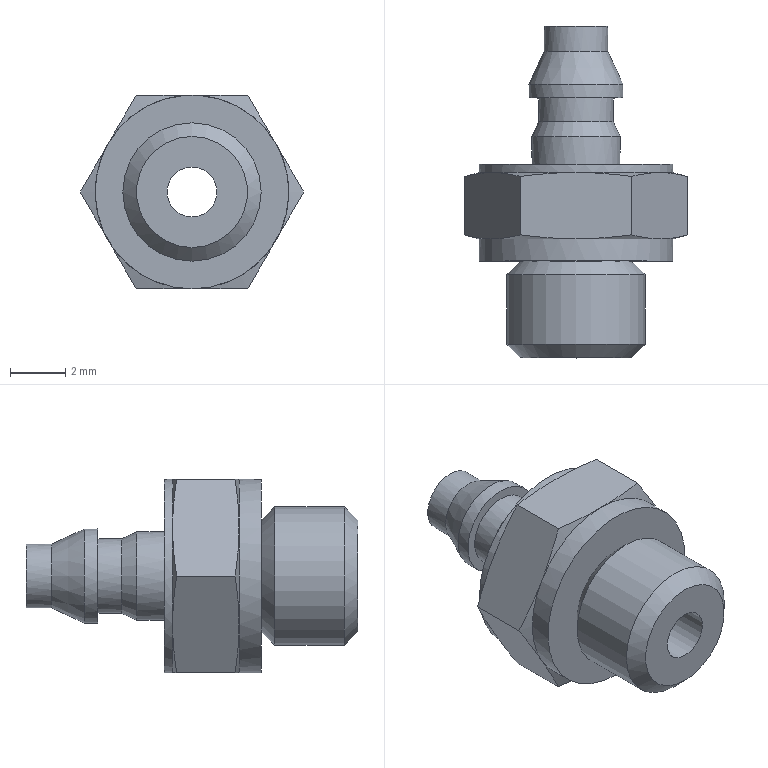Part | NX | 1 solid | 35 faces | box 8.083 x 12 x 7 mm | volume 211.126 mm3 | cone 16 | plane 11 | cylinder 8 | commonest cylinder face diameters 7 x2 1.8 x1 2.3 x1 2.7 x1 3.2 x1 3.4 x1
STEP:
#1=CARTESIAN_POINT('',(-3.031,3.2,-1.75));
#2=VERTEX_POINT('',#1);
#3=CARTESIAN_POINT('',(-3.031,3.2,1.75));
#4=VERTEX_POINT('',#3);
#5=CARTESIAN_POINT('',(0.,3.2,0.));
#6=DIRECTION('',(0.,-1.,0.));
#7=DIRECTION('',(-1.,0.,0.));
#8=AXIS2_PLACEMENT_3D('',#5,#6,#7);
#9=CIRCLE('',#8,3.5);
#10=EDGE_CURVE('',#2,#4,#9,.F.);
#11=ORIENTED_EDGE('',*,*,#10,.T.);
#12=CARTESIAN_POINT('',(0.,3.2,3.5));
#13=VERTEX_POINT('',#12);
#14=CARTESIAN_POINT('',(0.,3.2,0.));
#15=DIRECTION('',(0.,-1.,0.));
#16=DIRECTION('',(-1.,0.,0.));
#17=AXIS2_PLACEMENT_3D('',#14,#15,#16);
#18=CIRCLE('',#17,3.5);
#19=EDGE_CURVE('',#4,#13,#18,.F.);
#20=ORIENTED_EDGE('',*,*,#19,.T.);
#21=CARTESIAN_POINT('',(3.031,3.2,1.75));
#22=VERTEX_POINT('',#21);
#23=CARTESIAN_POINT('',(0.,3.2,0.));
#24=DIRECTION('',(0.,-1.,0.));
#25=DIRECTION('',(-1.,0.,0.));
#26=AXIS2_PLACEMENT_3D('',#23,#24,#25);
#27=CIRCLE('',#26,3.5);
#28=EDGE_CURVE('',#13,#22,#27,.F.);
#29=ORIENTED_EDGE('',*,*,#28,.T.);
#30=CARTESIAN_POINT('',(3.031,3.2,-1.75));
#31=VERTEX_POINT('',#30);
#32=CARTESIAN_POINT('',(0.,3.2,0.));
#33=DIRECTION('',(0.,-1.,0.));
#34=DIRECTION('',(-1.,0.,0.));
#35=AXIS2_PLACEMENT_3D('',#32,#33,#34);
#36=CIRCLE('',#35,3.5);
#37=EDGE_CURVE('',#22,#31,#36,.F.);
#38=ORIENTED_EDGE('',*,*,#37,.T.);
#39=CARTESIAN_POINT('',(0.,3.2,-3.5));
#40=VERTEX_POINT('',#39);
#41=CARTESIAN_POINT('',(0.,3.2,0.));
#42=DIRECTION('',(0.,-1.,0.));
#43=DIRECTION('',(-1.,0.,0.));
#44=AXIS2_PLACEMENT_3D('',#41,#42,#43);
#45=CIRCLE('',#44,3.5);
#46=EDGE_CURVE('',#31,#40,#45,.F.);
#47=ORIENTED_EDGE('',*,*,#46,.T.);
#48=CARTESIAN_POINT('',(0.,3.2,0.));
#49=DIRECTION('',(0.,-1.,0.));
#50=DIRECTION('',(-1.,0.,0.));
#51=AXIS2_PLACEMENT_3D('',#48,#49,#50);
#52=CIRCLE('',#51,3.5);
#53=EDGE_CURVE('',#40,#2,#52,.F.);
#54=ORIENTED_EDGE('',*,*,#53,.T.);
#55=EDGE_LOOP('',(#11,#20,#29,#38,#47,#54));
#56=FACE_BOUND('',#55,.T.);
#57=CARTESIAN_POINT('',(0.,3.5,-3.5));
#58=VERTEX_POINT('',#57);
#59=CARTESIAN_POINT('',(0.,3.5,0.));
#60=DIRECTION('',(0.,-1.,0.));
#61=DIRECTION('',(0.,0.,-1.));
#62=AXIS2_PLACEMENT_3D('',#59,#60,#61);
#63=CIRCLE('',#62,3.5);
#64=EDGE_CURVE('',#58,#58,#63,.T.);
#65=ORIENTED_EDGE('',*,*,#64,.T.);
#66=EDGE_LOOP('',(#65));
#67=FACE_BOUND('',#66,.T.);
#68=CARTESIAN_POINT('',(0.,3.2,0.));
#69=DIRECTION('',(0.,-1.,0.));
#70=DIRECTION('',(0.,0.,-1.));
#71=AXIS2_PLACEMENT_3D('',#68,#69,#70);
#72=CYLINDRICAL_SURFACE('',#71,3.5);
#73=ADVANCED_FACE('',(#56,#67),#72,.T.);
#74=ORIENTED_EDGE('',*,*,#10,.F.);
#75=CARTESIAN_POINT('',(-4.041,3.055,0.));
#76=VERTEX_POINT('',#75);
#77=CARTESIAN_POINT('',(-3.031,3.2,-1.75));
#78=CARTESIAN_POINT('',(-3.37,3.2,-1.164));
#79=CARTESIAN_POINT('',(-3.706,3.145,-0.5808));
#80=CARTESIAN_POINT('',(-4.041,3.055,0.));
#81=B_SPLINE_CURVE_WITH_KNOTS('',3,(#77,#78,#79,#80),.UNSPECIFIED.,.F.,.F.,(4,4),(0.,0.002026),.UNSPECIFIED.);
#82=EDGE_CURVE('',#2,#76,#81,.T.);
#83=ORIENTED_EDGE('',*,*,#82,.T.);
#84=CARTESIAN_POINT('',(-3.031,3.2,1.75));
#85=CARTESIAN_POINT('',(-3.37,3.2,1.164));
#86=CARTESIAN_POINT('',(-3.706,3.145,0.5808));
#87=CARTESIAN_POINT('',(-4.041,3.055,0.));
#88=B_SPLINE_CURVE_WITH_KNOTS('',3,(#84,#85,#86,#87),.UNSPECIFIED.,.F.,.F.,(4,4),(0.,0.002026),.UNSPECIFIED.);
#89=EDGE_CURVE('',#4,#76,#88,.T.);
#90=ORIENTED_EDGE('',*,*,#89,.F.);
#91=EDGE_LOOP('',(#74,#83,#90));
#92=FACE_BOUND('',#91,.T.);
#93=CARTESIAN_POINT('',(0.,3.2,0.));
#94=DIRECTION('',(0.,-1.,0.));
#95=DIRECTION('',(0.,0.,-1.));
#96=AXIS2_PLACEMENT_3D('',#93,#94,#95);
#97=CONICAL_SURFACE('',#96,3.5,1.309);
#98=ADVANCED_FACE('',(#92),#97,.T.);
#99=CARTESIAN_POINT('',(-2.021,3.055,-3.5));
#100=VERTEX_POINT('',#99);
#101=CARTESIAN_POINT('',(-2.021,3.055,-3.5));
#102=CARTESIAN_POINT('',(-2.356,3.145,-2.919));
#103=CARTESIAN_POINT('',(-2.693,3.2,-2.336));
#104=CARTESIAN_POINT('',(-3.031,3.2,-1.75));
#105=B_SPLINE_CURVE_WITH_KNOTS('',3,(#101,#102,#103,#104),.UNSPECIFIED.,.F.,.F.,(4,4),(0.,0.002026),.UNSPECIFIED.);
#106=EDGE_CURVE('',#100,#2,#105,.T.);
#107=ORIENTED_EDGE('',*,*,#106,.T.);
#108=ORIENTED_EDGE('',*,*,#53,.F.);
#109=CARTESIAN_POINT('',(0.,3.2,-3.5));
#110=CARTESIAN_POINT('',(-0.677,3.2,-3.5));
#111=CARTESIAN_POINT('',(-1.35,3.145,-3.5));
#112=CARTESIAN_POINT('',(-2.021,3.055,-3.5));
#113=B_SPLINE_CURVE_WITH_KNOTS('',3,(#109,#110,#111,#112),.UNSPECIFIED.,.F.,.F.,(4,4),(0.,0.002026),.UNSPECIFIED.);
#114=EDGE_CURVE('',#40,#100,#113,.T.);
#115=ORIENTED_EDGE('',*,*,#114,.T.);
#116=EDGE_LOOP('',(#107,#108,#115));
#117=FACE_BOUND('',#116,.T.);
#118=CARTESIAN_POINT('',(0.,3.2,0.));
#119=DIRECTION('',(0.,-1.,0.));
#120=DIRECTION('',(0.,0.,-1.));
#121=AXIS2_PLACEMENT_3D('',#118,#119,#120);
#122=CONICAL_SURFACE('',#121,3.5,1.309);
#123=ADVANCED_FACE('',(#117),#122,.T.);
#124=CARTESIAN_POINT('',(2.021,3.055,-3.5));
#125=VERTEX_POINT('',#124);
#126=CARTESIAN_POINT('',(2.021,3.055,-3.5));
#127=CARTESIAN_POINT('',(1.35,3.145,-3.5));
#128=CARTESIAN_POINT('',(0.677,3.2,-3.5));
#129=CARTESIAN_POINT('',(0.,3.2,-3.5));
#130=B_SPLINE_CURVE_WITH_KNOTS('',3,(#126,#127,#128,#129),.UNSPECIFIED.,.F.,.F.,(4,4),(0.,0.002026),.UNSPECIFIED.);
#131=EDGE_CURVE('',#125,#40,#130,.T.);
#132=ORIENTED_EDGE('',*,*,#131,.T.);
#133=ORIENTED_EDGE('',*,*,#46,.F.);
#134=CARTESIAN_POINT('',(3.031,3.2,-1.75));
#135=CARTESIAN_POINT('',(2.693,3.2,-2.336));
#136=CARTESIAN_POINT('',(2.356,3.145,-2.919));
#137=CARTESIAN_POINT('',(2.021,3.055,-3.5));
#138=B_SPLINE_CURVE_WITH_KNOTS('',3,(#134,#135,#136,#137),.UNSPECIFIED.,.F.,.F.,(4,4),(0.,0.002026),.UNSPECIFIED.);
#139=EDGE_CURVE('',#31,#125,#138,.T.);
#140=ORIENTED_EDGE('',*,*,#139,.T.);
#141=EDGE_LOOP('',(#132,#133,#140));
#142=FACE_BOUND('',#141,.T.);
#143=CARTESIAN_POINT('',(0.,3.2,0.));
#144=DIRECTION('',(0.,-1.,0.));
#145=DIRECTION('',(0.,0.,-1.));
#146=AXIS2_PLACEMENT_3D('',#143,#144,#145);
#147=CONICAL_SURFACE('',#146,3.5,1.309);
#148=ADVANCED_FACE('',(#142),#147,.T.);
#149=CARTESIAN_POINT('',(4.041,3.055,0.));
#150=VERTEX_POINT('',#149);
#151=CARTESIAN_POINT('',(4.041,3.055,0.));
#152=CARTESIAN_POINT('',(3.706,3.145,-0.5808));
#153=CARTESIAN_POINT('',(3.37,3.2,-1.164));
#154=CARTESIAN_POINT('',(3.031,3.2,-1.75));
#155=B_SPLINE_CURVE_WITH_KNOTS('',3,(#151,#152,#153,#154),.UNSPECIFIED.,.F.,.F.,(4,4),(0.,0.002026),.UNSPECIFIED.);
#156=EDGE_CURVE('',#150,#31,#155,.T.);
#157=ORIENTED_EDGE('',*,*,#156,.T.);
#158=ORIENTED_EDGE('',*,*,#37,.F.);
#159=CARTESIAN_POINT('',(4.041,3.055,0.));
#160=CARTESIAN_POINT('',(3.706,3.145,0.5808));
#161=CARTESIAN_POINT('',(3.37,3.2,1.164));
#162=CARTESIAN_POINT('',(3.031,3.2,1.75));
#163=B_SPLINE_CURVE_WITH_KNOTS('',3,(#159,#160,#161,#162),.UNSPECIFIED.,.F.,.F.,(4,4),(0.,0.002026),.UNSPECIFIED.);
#164=EDGE_CURVE('',#150,#22,#163,.T.);
#165=ORIENTED_EDGE('',*,*,#164,.F.);
#166=EDGE_LOOP('',(#157,#158,#165));
#167=FACE_BOUND('',#166,.T.);
#168=CARTESIAN_POINT('',(0.,3.2,0.));
#169=DIRECTION('',(0.,-1.,0.));
#170=DIRECTION('',(0.,0.,-1.));
#171=AXIS2_PLACEMENT_3D('',#168,#169,#170);
#172=CONICAL_SURFACE('',#171,3.5,1.309);
#173=ADVANCED_FACE('',(#167),#172,.T.);
#174=CARTESIAN_POINT('',(0.,3.5,-1.6));
#175=VERTEX_POINT('',#174);
#176=CARTESIAN_POINT('',(0.,3.5,0.));
#177=DIRECTION('',(0.,-1.,0.));
#178=DIRECTION('',(0.,0.,-1.));
#179=AXIS2_PLACEMENT_3D('',#176,#177,#178);
#180=CIRCLE('',#179,1.6);
#181=EDGE_CURVE('',#175,#175,#180,.T.);
#182=ORIENTED_EDGE('',*,*,#181,.T.);
#183=EDGE_LOOP('',(#182));
#184=FACE_BOUND('',#183,.T.);
#185=ORIENTED_EDGE('',*,*,#64,.F.);
#186=EDGE_LOOP('',(#185));
#187=FACE_BOUND('',#186,.T.);
#188=CARTESIAN_POINT('',(-3.5,3.5,3.542));
#189=DIRECTION('',(0.,1.,0.));
#190=DIRECTION('',(1.,0.,0.));
#191=AXIS2_PLACEMENT_3D('',#188,#189,#190);
#192=PLANE('',#191);
#193=ADVANCED_FACE('',(#184,#187),#192,.T.);
#194=CARTESIAN_POINT('',(-4.041,0.9451,0.));
#195=VERTEX_POINT('',#194);
#196=CARTESIAN_POINT('',(-4.041,0.8,0.));
#197=DIRECTION('',(0.,1.,0.));
#198=VECTOR('',#197,1000.);
#199=LINE('',#196,#198);
#200=EDGE_CURVE('',#195,#76,#199,.T.);
#201=ORIENTED_EDGE('',*,*,#200,.T.);
#202=ORIENTED_EDGE('',*,*,#82,.F.);
#203=ORIENTED_EDGE('',*,*,#106,.F.);
#204=CARTESIAN_POINT('',(-2.021,0.9451,-3.5));
#205=VERTEX_POINT('',#204);
#206=CARTESIAN_POINT('',(-2.021,0.8,-3.5));
#207=DIRECTION('',(0.,1.,0.));
#208=VECTOR('',#207,1000.);
#209=LINE('',#206,#208);
#210=EDGE_CURVE('',#100,#205,#209,.F.);
#211=ORIENTED_EDGE('',*,*,#210,.T.);
#212=CARTESIAN_POINT('',(-3.031,0.8,-1.75));
#213=VERTEX_POINT('',#212);
#214=CARTESIAN_POINT('',(-2.021,0.9451,-3.5));
#215=CARTESIAN_POINT('',(-2.356,0.8552,-2.919));
#216=CARTESIAN_POINT('',(-2.693,0.8,-2.336));
#217=CARTESIAN_POINT('',(-3.031,0.8,-1.75));
#218=B_SPLINE_CURVE_WITH_KNOTS('',3,(#214,#215,#216,#217),.UNSPECIFIED.,.F.,.F.,(4,4),(0.,0.002026),.UNSPECIFIED.);
#219=EDGE_CURVE('',#205,#213,#218,.T.);
#220=ORIENTED_EDGE('',*,*,#219,.T.);
#221=CARTESIAN_POINT('',(-3.031,0.8,-1.75));
#222=CARTESIAN_POINT('',(-3.37,0.8,-1.164));
#223=CARTESIAN_POINT('',(-3.706,0.8552,-0.5808));
#224=CARTESIAN_POINT('',(-4.041,0.9451,0.));
#225=B_SPLINE_CURVE_WITH_KNOTS('',3,(#221,#222,#223,#224),.UNSPECIFIED.,.F.,.F.,(4,4),(0.,0.002026),.UNSPECIFIED.);
#226=EDGE_CURVE('',#213,#195,#225,.T.);
#227=ORIENTED_EDGE('',*,*,#226,.T.);
#228=EDGE_LOOP('',(#201,#202,#203,#211,#220,#227));
#229=FACE_BOUND('',#228,.T.);
#230=CARTESIAN_POINT('',(-2.021,0.7856,-3.5));
#231=DIRECTION('',(-0.866,0.,-0.5));
#232=DIRECTION('',(-0.5,0.,0.866));
#233=AXIS2_PLACEMENT_3D('',#230,#231,#232);
#234=PLANE('',#233);
#235=ADVANCED_FACE('',(#229),#234,.T.);
#236=ORIENTED_EDGE('',*,*,#210,.F.);
#237=ORIENTED_EDGE('',*,*,#114,.F.);
#238=ORIENTED_EDGE('',*,*,#131,.F.);
#239=CARTESIAN_POINT('',(2.021,0.9451,-3.5));
#240=VERTEX_POINT('',#239);
#241=CARTESIAN_POINT('',(2.021,0.8,-3.5));
#242=DIRECTION('',(0.,1.,0.));
#243=VECTOR('',#242,1000.);
#244=LINE('',#241,#243);
#245=EDGE_CURVE('',#125,#240,#244,.F.);
#246=ORIENTED_EDGE('',*,*,#245,.T.);
#247=CARTESIAN_POINT('',(0.,0.8,-3.5));
#248=VERTEX_POINT('',#247);
#249=CARTESIAN_POINT('',(2.021,0.9451,-3.5));
#250=CARTESIAN_POINT('',(1.35,0.8552,-3.5));
#251=CARTESIAN_POINT('',(0.677,0.8,-3.5));
#252=CARTESIAN_POINT('',(0.,0.8,-3.5));
#253=B_SPLINE_CURVE_WITH_KNOTS('',3,(#249,#250,#251,#252),.UNSPECIFIED.,.F.,.F.,(4,4),(0.,0.002026),.UNSPECIFIED.);
#254=EDGE_CURVE('',#240,#248,#253,.T.);
#255=ORIENTED_EDGE('',*,*,#254,.T.);
#256=CARTESIAN_POINT('',(0.,0.8,-3.5));
#257=CARTESIAN_POINT('',(-0.677,0.8,-3.5));
#258=CARTESIAN_POINT('',(-1.35,0.8552,-3.5));
#259=CARTESIAN_POINT('',(-2.021,0.9451,-3.5));
#260=B_SPLINE_CURVE_WITH_KNOTS('',3,(#256,#257,#258,#259),.UNSPECIFIED.,.F.,.F.,(4,4),(0.,0.002026),.UNSPECIFIED.);
#261=EDGE_CURVE('',#248,#205,#260,.T.);
#262=ORIENTED_EDGE('',*,*,#261,.T.);
#263=EDGE_LOOP('',(#236,#237,#238,#246,#255,#262));
#264=FACE_BOUND('',#263,.T.);
#265=CARTESIAN_POINT('',(2.021,0.7856,-3.5));
#266=DIRECTION('',(0.,0.,-1.));
#267=DIRECTION('',(-1.,0.,0.));
#268=AXIS2_PLACEMENT_3D('',#265,#266,#267);
#269=PLANE('',#268);
#270=ADVANCED_FACE('',(#264),#269,.T.);
#271=ORIENTED_EDGE('',*,*,#245,.F.);
#272=ORIENTED_EDGE('',*,*,#139,.F.);
#273=ORIENTED_EDGE('',*,*,#156,.F.);
#274=CARTESIAN_POINT('',(4.041,0.9451,0.));
#275=VERTEX_POINT('',#274);
#276=CARTESIAN_POINT('',(4.041,0.8,0.));
#277=DIRECTION('',(0.,1.,0.));
#278=VECTOR('',#277,1000.);
#279=LINE('',#276,#278);
#280=EDGE_CURVE('',#150,#275,#279,.F.);
#281=ORIENTED_EDGE('',*,*,#280,.T.);
#282=CARTESIAN_POINT('',(3.031,0.8,-1.75));
#283=VERTEX_POINT('',#282);
#284=CARTESIAN_POINT('',(4.041,0.9451,0.));
#285=CARTESIAN_POINT('',(3.706,0.8552,-0.5808));
#286=CARTESIAN_POINT('',(3.37,0.8,-1.164));
#287=CARTESIAN_POINT('',(3.031,0.8,-1.75));
#288=B_SPLINE_CURVE_WITH_KNOTS('',3,(#284,#285,#286,#287),.UNSPECIFIED.,.F.,.F.,(4,4),(0.,0.002026),.UNSPECIFIED.);
#289=EDGE_CURVE('',#275,#283,#288,.T.);
#290=ORIENTED_EDGE('',*,*,#289,.T.);
#291=CARTESIAN_POINT('',(3.031,0.8,-1.75));
#292=CARTESIAN_POINT('',(2.693,0.8,-2.336));
#293=CARTESIAN_POINT('',(2.356,0.8552,-2.919));
#294=CARTESIAN_POINT('',(2.021,0.9451,-3.5));
#295=B_SPLINE_CURVE_WITH_KNOTS('',3,(#291,#292,#293,#294),.UNSPECIFIED.,.F.,.F.,(4,4),(0.,0.002026),.UNSPECIFIED.);
#296=EDGE_CURVE('',#283,#240,#295,.T.);
#297=ORIENTED_EDGE('',*,*,#296,.T.);
#298=EDGE_LOOP('',(#271,#272,#273,#281,#290,#297));
#299=FACE_BOUND('',#298,.T.);
#300=CARTESIAN_POINT('',(4.041,0.7856,0.));
#301=DIRECTION('',(0.866,0.,-0.5));
#302=DIRECTION('',(-0.5,0.,-0.866));
#303=AXIS2_PLACEMENT_3D('',#300,#301,#302);
#304=PLANE('',#303);
#305=ADVANCED_FACE('',(#299),#304,.T.);
#306=ORIENTED_EDGE('',*,*,#181,.F.);
#307=EDGE_LOOP('',(#306));
#308=FACE_BOUND('',#307,.T.);
#309=CARTESIAN_POINT('',(-1.6,4.5,0.));
#310=VERTEX_POINT('',#309);
#311=CARTESIAN_POINT('',(0.,4.5,0.));
#312=DIRECTION('',(0.,-1.,0.));
#313=DIRECTION('',(-1.,0.,0.));
#314=AXIS2_PLACEMENT_3D('',#311,#312,#313);
#315=CIRCLE('',#314,1.6);
#316=EDGE_CURVE('',#310,#310,#315,.T.);
#317=ORIENTED_EDGE('',*,*,#316,.T.);
#318=EDGE_LOOP('',(#317));
#319=FACE_BOUND('',#318,.T.);
#320=CARTESIAN_POINT('',(0.,3.5,0.));
#321=DIRECTION('',(0.,-1.,0.));
#322=DIRECTION('',(0.,0.,-1.));
#323=AXIS2_PLACEMENT_3D('',#320,#321,#322);
#324=CYLINDRICAL_SURFACE('',#323,1.6);
#325=ADVANCED_FACE('',(#308,#319),#324,.T.);
#326=CARTESIAN_POINT('',(-3.031,0.8,1.75));
#327=VERTEX_POINT('',#326);
#328=CARTESIAN_POINT('',(-2.021,0.9451,3.5));
#329=VERTEX_POINT('',#328);
#330=CARTESIAN_POINT('',(-3.031,0.8,1.75));
#331=CARTESIAN_POINT('',(-2.693,0.8,2.336));
#332=CARTESIAN_POINT('',(-2.356,0.8552,2.919));
#333=CARTESIAN_POINT('',(-2.021,0.9451,3.5));
#334=B_SPLINE_CURVE_WITH_KNOTS('',3,(#330,#331,#332,#333),.UNSPECIFIED.,.F.,.F.,(4,4),(0.,0.002026),.UNSPECIFIED.);
#335=EDGE_CURVE('',#327,#329,#334,.T.);
#336=ORIENTED_EDGE('',*,*,#335,.T.);
#337=CARTESIAN_POINT('',(-2.021,3.055,3.5));
#338=VERTEX_POINT('',#337);
#339=CARTESIAN_POINT('',(-2.021,0.8,3.5));
#340=DIRECTION('',(0.,1.,0.));
#341=VECTOR('',#340,1000.);
#342=LINE('',#339,#341);
#343=EDGE_CURVE('',#329,#338,#342,.T.);
#344=ORIENTED_EDGE('',*,*,#343,.T.);
#345=CARTESIAN_POINT('',(-2.021,3.055,3.5));
#346=CARTESIAN_POINT('',(-2.356,3.145,2.919));
#347=CARTESIAN_POINT('',(-2.693,3.2,2.336));
#348=CARTESIAN_POINT('',(-3.031,3.2,1.75));
#349=B_SPLINE_CURVE_WITH_KNOTS('',3,(#345,#346,#347,#348),.UNSPECIFIED.,.F.,.F.,(4,4),(0.,0.002026),.UNSPECIFIED.);
#350=EDGE_CURVE('',#338,#4,#349,.T.);
#351=ORIENTED_EDGE('',*,*,#350,.T.);
#352=ORIENTED_EDGE('',*,*,#89,.T.);
#353=ORIENTED_EDGE('',*,*,#200,.F.);
#354=CARTESIAN_POINT('',(-4.041,0.9451,0.));
#355=CARTESIAN_POINT('',(-3.706,0.8552,0.5808));
#356=CARTESIAN_POINT('',(-3.37,0.8,1.164));
#357=CARTESIAN_POINT('',(-3.031,0.8,1.75));
#358=B_SPLINE_CURVE_WITH_KNOTS('',3,(#354,#355,#356,#357),.UNSPECIFIED.,.F.,.F.,(4,4),(0.,0.002026),.UNSPECIFIED.);
#359=EDGE_CURVE('',#195,#327,#358,.T.);
#360=ORIENTED_EDGE('',*,*,#359,.T.);
#361=EDGE_LOOP('',(#336,#344,#351,#352,#353,#360));
#362=FACE_BOUND('',#361,.T.);
#363=CARTESIAN_POINT('',(-4.041,0.7856,0.));
#364=DIRECTION('',(-0.866,0.,0.5));
#365=DIRECTION('',(0.5,0.,0.866));
#366=AXIS2_PLACEMENT_3D('',#363,#364,#365);
#367=PLANE('',#366);
#368=ADVANCED_FACE('',(#362),#367,.T.);
#369=ORIENTED_EDGE('',*,*,#226,.F.);
#370=CARTESIAN_POINT('',(0.,0.8,0.));
#371=DIRECTION('',(0.,-1.,0.));
#372=DIRECTION('',(-1.,0.,0.));
#373=AXIS2_PLACEMENT_3D('',#370,#371,#372);
#374=CIRCLE('',#373,3.5);
#375=EDGE_CURVE('',#213,#327,#374,.F.);
#376=ORIENTED_EDGE('',*,*,#375,.T.);
#377=ORIENTED_EDGE('',*,*,#359,.F.);
#378=EDGE_LOOP('',(#369,#376,#377));
#379=FACE_BOUND('',#378,.T.);
#380=CARTESIAN_POINT('',(0.,0.8,0.));
#381=DIRECTION('',(0.,1.,0.));
#382=DIRECTION('',(0.,0.,1.));
#383=AXIS2_PLACEMENT_3D('',#380,#381,#382);
#384=CONICAL_SURFACE('',#383,3.5,1.309);
#385=ADVANCED_FACE('',(#379),#384,.T.);
#386=ORIENTED_EDGE('',*,*,#261,.F.);
#387=CARTESIAN_POINT('',(0.,0.8,0.));
#388=DIRECTION('',(0.,-1.,0.));
#389=DIRECTION('',(-1.,0.,0.));
#390=AXIS2_PLACEMENT_3D('',#387,#388,#389);
#391=CIRCLE('',#390,3.5);
#392=EDGE_CURVE('',#248,#213,#391,.F.);
#393=ORIENTED_EDGE('',*,*,#392,.T.);
#394=ORIENTED_EDGE('',*,*,#219,.F.);
#395=EDGE_LOOP('',(#386,#393,#394));
#396=FACE_BOUND('',#395,.T.);
#397=CARTESIAN_POINT('',(0.,0.8,0.));
#398=DIRECTION('',(0.,1.,0.));
#399=DIRECTION('',(0.,0.,1.));
#400=AXIS2_PLACEMENT_3D('',#397,#398,#399);
#401=CONICAL_SURFACE('',#400,3.5,1.309);
#402=ADVANCED_FACE('',(#396),#401,.T.);
#403=CARTESIAN_POINT('',(0.,0.8,0.));
#404=DIRECTION('',(0.,-1.,0.));
#405=DIRECTION('',(-1.,0.,0.));
#406=AXIS2_PLACEMENT_3D('',#403,#404,#405);
#407=CIRCLE('',#406,3.5);
#408=EDGE_CURVE('',#283,#248,#407,.F.);
#409=ORIENTED_EDGE('',*,*,#408,.T.);
#410=ORIENTED_EDGE('',*,*,#254,.F.);
#411=ORIENTED_EDGE('',*,*,#296,.F.);
#412=EDGE_LOOP('',(#409,#410,#411));
#413=FACE_BOUND('',#412,.T.);
#414=CARTESIAN_POINT('',(0.,0.8,0.));
#415=DIRECTION('',(0.,1.,0.));
#416=DIRECTION('',(0.,0.,1.));
#417=AXIS2_PLACEMENT_3D('',#414,#415,#416);
#418=CONICAL_SURFACE('',#417,3.5,1.309);
#419=ADVANCED_FACE('',(#413),#418,.T.);
#420=CARTESIAN_POINT('',(3.031,0.8,1.75));
#421=VERTEX_POINT('',#420);
#422=CARTESIAN_POINT('',(0.,0.8,0.));
#423=DIRECTION('',(0.,-1.,0.));
#424=DIRECTION('',(-1.,0.,0.));
#425=AXIS2_PLACEMENT_3D('',#422,#423,#424);
#426=CIRCLE('',#425,3.5);
#427=EDGE_CURVE('',#421,#283,#426,.F.);
#428=ORIENTED_EDGE('',*,*,#427,.T.);
#429=ORIENTED_EDGE('',*,*,#289,.F.);
#430=CARTESIAN_POINT('',(3.031,0.8,1.75));
#431=CARTESIAN_POINT('',(3.37,0.8,1.164));
#432=CARTESIAN_POINT('',(3.706,0.8552,0.5808));
#433=CARTESIAN_POINT('',(4.041,0.9451,0.));
#434=B_SPLINE_CURVE_WITH_KNOTS('',3,(#430,#431,#432,#433),.UNSPECIFIED.,.F.,.F.,(4,4),(0.,0.002026),.UNSPECIFIED.);
#435=EDGE_CURVE('',#421,#275,#434,.T.);
#436=ORIENTED_EDGE('',*,*,#435,.F.);
#437=EDGE_LOOP('',(#428,#429,#436));
#438=FACE_BOUND('',#437,.T.);
#439=CARTESIAN_POINT('',(0.,0.8,0.));
#440=DIRECTION('',(0.,1.,0.));
#441=DIRECTION('',(0.,0.,1.));
#442=AXIS2_PLACEMENT_3D('',#439,#440,#441);
#443=CONICAL_SURFACE('',#442,3.5,1.309);
#444=ADVANCED_FACE('',(#438),#443,.T.);
#445=ORIENTED_EDGE('',*,*,#435,.T.);
#446=ORIENTED_EDGE('',*,*,#280,.F.);
#447=ORIENTED_EDGE('',*,*,#164,.T.);
#448=CARTESIAN_POINT('',(2.021,3.055,3.5));
#449=VERTEX_POINT('',#448);
#450=CARTESIAN_POINT('',(3.031,3.2,1.75));
#451=CARTESIAN_POINT('',(2.693,3.2,2.336));
#452=CARTESIAN_POINT('',(2.356,3.145,2.919));
#453=CARTESIAN_POINT('',(2.021,3.055,3.5));
#454=B_SPLINE_CURVE_WITH_KNOTS('',3,(#450,#451,#452,#453),.UNSPECIFIED.,.F.,.F.,(4,4),(0.,0.002026),.UNSPECIFIED.);
#455=EDGE_CURVE('',#22,#449,#454,.T.);
#456=ORIENTED_EDGE('',*,*,#455,.T.);
#457=CARTESIAN_POINT('',(2.021,0.9451,3.5));
#458=VERTEX_POINT('',#457);
#459=CARTESIAN_POINT('',(2.021,0.8,3.5));
#460=DIRECTION('',(0.,1.,0.));
#461=VECTOR('',#460,1000.);
#462=LINE('',#459,#461);
#463=EDGE_CURVE('',#449,#458,#462,.F.);
#464=ORIENTED_EDGE('',*,*,#463,.T.);
#465=CARTESIAN_POINT('',(2.021,0.9451,3.5));
#466=CARTESIAN_POINT('',(2.356,0.8552,2.919));
#467=CARTESIAN_POINT('',(2.693,0.8,2.336));
#468=CARTESIAN_POINT('',(3.031,0.8,1.75));
#469=B_SPLINE_CURVE_WITH_KNOTS('',3,(#465,#466,#467,#468),.UNSPECIFIED.,.F.,.F.,(4,4),(0.,0.002026),.UNSPECIFIED.);
#470=EDGE_CURVE('',#458,#421,#469,.T.);
#471=ORIENTED_EDGE('',*,*,#470,.T.);
#472=EDGE_LOOP('',(#445,#446,#447,#456,#464,#471));
#473=FACE_BOUND('',#472,.T.);
#474=CARTESIAN_POINT('',(2.021,0.7856,3.5));
#475=DIRECTION('',(0.866,0.,0.5));
#476=DIRECTION('',(0.5,0.,-0.866));
#477=AXIS2_PLACEMENT_3D('',#474,#475,#476);
#478=PLANE('',#477);
#479=ADVANCED_FACE('',(#473),#478,.T.);
#480=ORIENTED_EDGE('',*,*,#316,.F.);
#481=EDGE_LOOP('',(#480));
#482=FACE_BOUND('',#481,.T.);
#483=CARTESIAN_POINT('',(-1.35,5.04,0.));
#484=VERTEX_POINT('',#483);
#485=CARTESIAN_POINT('',(0.,5.04,0.));
#486=DIRECTION('',(0.,1.,0.));
#487=DIRECTION('',(-1.,0.,0.));
#488=AXIS2_PLACEMENT_3D('',#485,#486,#487);
#489=CIRCLE('',#488,1.35);
#490=EDGE_CURVE('',#484,#484,#489,.F.);
#491=ORIENTED_EDGE('',*,*,#490,.T.);
#492=EDGE_LOOP('',(#491));
#493=FACE_BOUND('',#492,.T.);
#494=CARTESIAN_POINT('',(0.,5.04,0.));
#495=DIRECTION('',(0.,-1.,0.));
#496=DIRECTION('',(0.,0.,-1.));
#497=AXIS2_PLACEMENT_3D('',#494,#495,#496);
#498=CONICAL_SURFACE('',#497,1.35,0.4336);
#499=ADVANCED_FACE('',(#482,#493),#498,.T.);
#500=ORIENTED_EDGE('',*,*,#28,.F.);
#501=CARTESIAN_POINT('',(0.,3.2,3.5));
#502=CARTESIAN_POINT('',(0.677,3.2,3.5));
#503=CARTESIAN_POINT('',(1.35,3.145,3.5));
#504=CARTESIAN_POINT('',(2.021,3.055,3.5));
#505=B_SPLINE_CURVE_WITH_KNOTS('',3,(#501,#502,#503,#504),.UNSPECIFIED.,.F.,.F.,(4,4),(0.,0.002026),.UNSPECIFIED.);
#506=EDGE_CURVE('',#13,#449,#505,.T.);
#507=ORIENTED_EDGE('',*,*,#506,.T.);
#508=ORIENTED_EDGE('',*,*,#455,.F.);
#509=EDGE_LOOP('',(#500,#507,#508));
#510=FACE_BOUND('',#509,.T.);
#511=CARTESIAN_POINT('',(0.,3.2,0.));
#512=DIRECTION('',(0.,-1.,0.));
#513=DIRECTION('',(0.,0.,-1.));
#514=AXIS2_PLACEMENT_3D('',#511,#512,#513);
#515=CONICAL_SURFACE('',#514,3.5,1.309);
#516=ADVANCED_FACE('',(#510),#515,.T.);
#517=ORIENTED_EDGE('',*,*,#19,.F.);
#518=ORIENTED_EDGE('',*,*,#350,.F.);
#519=CARTESIAN_POINT('',(-2.021,3.055,3.5));
#520=CARTESIAN_POINT('',(-1.35,3.145,3.5));
#521=CARTESIAN_POINT('',(-0.677,3.2,3.5));
#522=CARTESIAN_POINT('',(0.,3.2,3.5));
#523=B_SPLINE_CURVE_WITH_KNOTS('',3,(#519,#520,#521,#522),.UNSPECIFIED.,.F.,.F.,(4,4),(0.,0.002026),.UNSPECIFIED.);
#524=EDGE_CURVE('',#338,#13,#523,.T.);
#525=ORIENTED_EDGE('',*,*,#524,.T.);
#526=EDGE_LOOP('',(#517,#518,#525));
#527=FACE_BOUND('',#526,.T.);
#528=CARTESIAN_POINT('',(0.,3.2,0.));
#529=DIRECTION('',(0.,-1.,0.));
#530=DIRECTION('',(0.,0.,-1.));
#531=AXIS2_PLACEMENT_3D('',#528,#529,#530);
#532=CONICAL_SURFACE('',#531,3.5,1.309);
#533=ADVANCED_FACE('',(#527),#532,.T.);
#534=CARTESIAN_POINT('',(0.,0.8,3.5));
#535=VERTEX_POINT('',#534);
#536=CARTESIAN_POINT('',(0.,0.8,3.5));
#537=CARTESIAN_POINT('',(0.677,0.8,3.5));
#538=CARTESIAN_POINT('',(1.35,0.8552,3.5));
#539=CARTESIAN_POINT('',(2.021,0.9451,3.5));
#540=B_SPLINE_CURVE_WITH_KNOTS('',3,(#536,#537,#538,#539),.UNSPECIFIED.,.F.,.F.,(4,4),(0.,0.002026),.UNSPECIFIED.);
#541=EDGE_CURVE('',#535,#458,#540,.T.);
#542=ORIENTED_EDGE('',*,*,#541,.T.);
#543=ORIENTED_EDGE('',*,*,#463,.F.);
#544=ORIENTED_EDGE('',*,*,#506,.F.);
#545=ORIENTED_EDGE('',*,*,#524,.F.);
#546=ORIENTED_EDGE('',*,*,#343,.F.);
#547=CARTESIAN_POINT('',(-2.021,0.9451,3.5));
#548=CARTESIAN_POINT('',(-1.35,0.8552,3.5));
#549=CARTESIAN_POINT('',(-0.677,0.8,3.5));
#550=CARTESIAN_POINT('',(0.,0.8,3.5));
#551=B_SPLINE_CURVE_WITH_KNOTS('',3,(#547,#548,#549,#550),.UNSPECIFIED.,.F.,.F.,(4,4),(0.,0.002026),.UNSPECIFIED.);
#552=EDGE_CURVE('',#329,#535,#551,.T.);
#553=ORIENTED_EDGE('',*,*,#552,.T.);
#554=EDGE_LOOP('',(#542,#543,#544,#545,#546,#553));
#555=FACE_BOUND('',#554,.T.);
#556=CARTESIAN_POINT('',(-2.021,0.7856,3.5));
#557=DIRECTION('',(0.,0.,1.));
#558=DIRECTION('',(1.,0.,0.));
#559=AXIS2_PLACEMENT_3D('',#556,#557,#558);
#560=PLANE('',#559);
#561=ADVANCED_FACE('',(#555),#560,.T.);
#562=ORIENTED_EDGE('',*,*,#335,.F.);
#563=CARTESIAN_POINT('',(0.,0.8,0.));
#564=DIRECTION('',(0.,-1.,0.));
#565=DIRECTION('',(-1.,0.,0.));
#566=AXIS2_PLACEMENT_3D('',#563,#564,#565);
#567=CIRCLE('',#566,3.5);
#568=EDGE_CURVE('',#327,#535,#567,.F.);
#569=ORIENTED_EDGE('',*,*,#568,.T.);
#570=ORIENTED_EDGE('',*,*,#552,.F.);
#571=EDGE_LOOP('',(#562,#569,#570));
#572=FACE_BOUND('',#571,.T.);
#573=CARTESIAN_POINT('',(0.,0.8,0.));
#574=DIRECTION('',(0.,1.,0.));
#575=DIRECTION('',(0.,0.,1.));
#576=AXIS2_PLACEMENT_3D('',#573,#574,#575);
#577=CONICAL_SURFACE('',#576,3.5,1.309);
#578=ADVANCED_FACE('',(#572),#577,.T.);
#579=ORIENTED_EDGE('',*,*,#568,.F.);
#580=ORIENTED_EDGE('',*,*,#375,.F.);
#581=ORIENTED_EDGE('',*,*,#392,.F.);
#582=ORIENTED_EDGE('',*,*,#408,.F.);
#583=ORIENTED_EDGE('',*,*,#427,.F.);
#584=CARTESIAN_POINT('',(0.,0.8,0.));
#585=DIRECTION('',(0.,-1.,0.));
#586=DIRECTION('',(-1.,0.,0.));
#587=AXIS2_PLACEMENT_3D('',#584,#585,#586);
#588=CIRCLE('',#587,3.5);
#589=EDGE_CURVE('',#535,#421,#588,.F.);
#590=ORIENTED_EDGE('',*,*,#589,.F.);
#591=EDGE_LOOP('',(#579,#580,#581,#582,#583,#590));
#592=FACE_BOUND('',#591,.T.);
#593=CARTESIAN_POINT('',(0.,0.,-3.5));
#594=VERTEX_POINT('',#593);
#595=CARTESIAN_POINT('',(0.,0.,0.));
#596=DIRECTION('',(0.,-1.,0.));
#597=DIRECTION('',(0.,0.,-1.));
#598=AXIS2_PLACEMENT_3D('',#595,#596,#597);
#599=CIRCLE('',#598,3.5);
#600=EDGE_CURVE('',#594,#594,#599,.F.);
#601=ORIENTED_EDGE('',*,*,#600,.T.);
#602=EDGE_LOOP('',(#601));
#603=FACE_BOUND('',#602,.T.);
#604=CARTESIAN_POINT('',(0.,0.,0.));
#605=DIRECTION('',(0.,-1.,0.));
#606=DIRECTION('',(0.,0.,-1.));
#607=AXIS2_PLACEMENT_3D('',#604,#605,#606);
#608=CYLINDRICAL_SURFACE('',#607,3.5);
#609=ADVANCED_FACE('',(#592,#603),#608,.T.);
#610=ORIENTED_EDGE('',*,*,#589,.T.);
#611=ORIENTED_EDGE('',*,*,#470,.F.);
#612=ORIENTED_EDGE('',*,*,#541,.F.);
#613=EDGE_LOOP('',(#610,#611,#612));
#614=FACE_BOUND('',#613,.T.);
#615=CARTESIAN_POINT('',(0.,0.8,0.));
#616=DIRECTION('',(0.,1.,0.));
#617=DIRECTION('',(0.,0.,1.));
#618=AXIS2_PLACEMENT_3D('',#615,#616,#617);
#619=CONICAL_SURFACE('',#618,3.5,1.309);
#620=ADVANCED_FACE('',(#614),#619,.T.);
#621=ORIENTED_EDGE('',*,*,#490,.F.);
#622=EDGE_LOOP('',(#621));
#623=FACE_BOUND('',#622,.T.);
#624=CARTESIAN_POINT('',(0.,5.9,-1.35));
#625=VERTEX_POINT('',#624);
#626=CARTESIAN_POINT('',(0.,5.9,0.));
#627=DIRECTION('',(0.,-1.,0.));
#628=DIRECTION('',(0.,0.,-1.));
#629=AXIS2_PLACEMENT_3D('',#626,#627,#628);
#630=CIRCLE('',#629,1.35);
#631=EDGE_CURVE('',#625,#625,#630,.T.);
#632=ORIENTED_EDGE('',*,*,#631,.T.);
#633=EDGE_LOOP('',(#632));
#634=FACE_BOUND('',#633,.T.);
#635=CARTESIAN_POINT('',(0.,5.04,0.));
#636=DIRECTION('',(0.,-1.,0.));
#637=DIRECTION('',(0.,0.,-1.));
#638=AXIS2_PLACEMENT_3D('',#635,#636,#637);
#639=CYLINDRICAL_SURFACE('',#638,1.35);
#640=ADVANCED_FACE('',(#623,#634),#639,.T.);
#641=CARTESIAN_POINT('',(0.,0.,-2.01));
#642=VERTEX_POINT('',#641);
#643=CARTESIAN_POINT('',(0.,0.,0.));
#644=DIRECTION('',(0.,-1.,0.));
#645=DIRECTION('',(0.,0.,-1.));
#646=AXIS2_PLACEMENT_3D('',#643,#644,#645);
#647=CIRCLE('',#646,2.01);
#648=EDGE_CURVE('',#642,#642,#647,.F.);
#649=ORIENTED_EDGE('',*,*,#648,.T.);
#650=EDGE_LOOP('',(#649));
#651=FACE_BOUND('',#650,.T.);
#652=ORIENTED_EDGE('',*,*,#600,.F.);
#653=EDGE_LOOP('',(#652));
#654=FACE_BOUND('',#653,.T.);
#655=CARTESIAN_POINT('',(3.5,0.,3.542));
#656=DIRECTION('',(0.,-1.,0.));
#657=DIRECTION('',(-1.,0.,0.));
#658=AXIS2_PLACEMENT_3D('',#655,#656,#657);
#659=PLANE('',#658);
#660=ADVANCED_FACE('',(#651,#654),#659,.T.);
#661=ORIENTED_EDGE('',*,*,#631,.F.);
#662=EDGE_LOOP('',(#661));
#663=FACE_BOUND('',#662,.T.);
#664=CARTESIAN_POINT('',(0.,5.9,-1.7));
#665=VERTEX_POINT('',#664);
#666=CARTESIAN_POINT('',(0.,5.9,0.));
#667=DIRECTION('',(0.,-1.,0.));
#668=DIRECTION('',(0.,0.,-1.));
#669=AXIS2_PLACEMENT_3D('',#666,#667,#668);
#670=CIRCLE('',#669,1.7);
#671=EDGE_CURVE('',#665,#665,#670,.T.);
#672=ORIENTED_EDGE('',*,*,#671,.T.);
#673=EDGE_LOOP('',(#672));
#674=FACE_BOUND('',#673,.T.);
#675=CARTESIAN_POINT('',(1.7,5.9,1.72));
#676=DIRECTION('',(0.,-1.,0.));
#677=DIRECTION('',(-1.,0.,0.));
#678=AXIS2_PLACEMENT_3D('',#675,#676,#677);
#679=PLANE('',#678);
#680=ADVANCED_FACE('',(#663,#674),#679,.T.);
#681=CARTESIAN_POINT('',(-2.5,-0.4905,0.));
#682=VERTEX_POINT('',#681);
#683=CARTESIAN_POINT('',(0.,-0.4905,0.));
#684=DIRECTION('',(0.,1.,0.));
#685=DIRECTION('',(-1.,0.,0.));
#686=AXIS2_PLACEMENT_3D('',#683,#684,#685);
#687=CIRCLE('',#686,2.5);
#688=EDGE_CURVE('',#682,#682,#687,.T.);
#689=ORIENTED_EDGE('',*,*,#688,.T.);
#690=EDGE_LOOP('',(#689));
#691=FACE_BOUND('',#690,.T.);
#692=ORIENTED_EDGE('',*,*,#648,.F.);
#693=EDGE_LOOP('',(#692));
#694=FACE_BOUND('',#693,.T.);
#695=CARTESIAN_POINT('',(0.,0.,0.));
#696=DIRECTION('',(0.,-1.,0.));
#697=DIRECTION('',(0.,0.,-1.));
#698=AXIS2_PLACEMENT_3D('',#695,#696,#697);
#699=CONICAL_SURFACE('',#698,2.01,0.7854);
#700=ADVANCED_FACE('',(#691,#694),#699,.T.);
#701=ORIENTED_EDGE('',*,*,#671,.F.);
#702=EDGE_LOOP('',(#701));
#703=FACE_BOUND('',#702,.T.);
#704=CARTESIAN_POINT('',(-1.7,6.4,0.));
#705=VERTEX_POINT('',#704);
#706=CARTESIAN_POINT('',(0.,6.4,0.));
#707=DIRECTION('',(0.,-1.,0.));
#708=DIRECTION('',(-1.,0.,0.));
#709=AXIS2_PLACEMENT_3D('',#706,#707,#708);
#710=CIRCLE('',#709,1.7);
#711=EDGE_CURVE('',#705,#705,#710,.T.);
#712=ORIENTED_EDGE('',*,*,#711,.T.);
#713=EDGE_LOOP('',(#712));
#714=FACE_BOUND('',#713,.T.);
#715=CARTESIAN_POINT('',(0.,5.9,0.));
#716=DIRECTION('',(0.,-1.,0.));
#717=DIRECTION('',(0.,0.,-1.));
#718=AXIS2_PLACEMENT_3D('',#715,#716,#717);
#719=CYLINDRICAL_SURFACE('',#718,1.7);
#720=ADVANCED_FACE('',(#703,#714),#719,.T.);
#721=CARTESIAN_POINT('',(-2.5,-3.01,0.));
#722=VERTEX_POINT('',#721);
#723=CARTESIAN_POINT('',(0.,-3.01,0.));
#724=DIRECTION('',(0.,-1.,0.));
#725=DIRECTION('',(-1.,0.,0.));
#726=AXIS2_PLACEMENT_3D('',#723,#724,#725);
#727=CIRCLE('',#726,2.5);
#728=EDGE_CURVE('',#722,#722,#727,.F.);
#729=ORIENTED_EDGE('',*,*,#728,.T.);
#730=EDGE_LOOP('',(#729));
#731=FACE_BOUND('',#730,.T.);
#732=ORIENTED_EDGE('',*,*,#688,.F.);
#733=EDGE_LOOP('',(#732));
#734=FACE_BOUND('',#733,.T.);
#735=CARTESIAN_POINT('',(0.,-3.01,0.));
#736=DIRECTION('',(0.,-1.,0.));
#737=DIRECTION('',(0.,0.,-1.));
#738=AXIS2_PLACEMENT_3D('',#735,#736,#737);
#739=CYLINDRICAL_SURFACE('',#738,2.5);
#740=ADVANCED_FACE('',(#731,#734),#739,.T.);
#741=ORIENTED_EDGE('',*,*,#711,.F.);
#742=EDGE_LOOP('',(#741));
#743=FACE_BOUND('',#742,.T.);
#744=CARTESIAN_POINT('',(-1.15,7.58,0.));
#745=VERTEX_POINT('',#744);
#746=CARTESIAN_POINT('',(0.,7.58,0.));
#747=DIRECTION('',(0.,1.,0.));
#748=DIRECTION('',(-1.,0.,0.));
#749=AXIS2_PLACEMENT_3D('',#746,#747,#748);
#750=CIRCLE('',#749,1.15);
#751=EDGE_CURVE('',#745,#745,#750,.F.);
#752=ORIENTED_EDGE('',*,*,#751,.T.);
#753=EDGE_LOOP('',(#752));
#754=FACE_BOUND('',#753,.T.);
#755=CARTESIAN_POINT('',(0.,7.58,0.));
#756=DIRECTION('',(0.,-1.,0.));
#757=DIRECTION('',(0.,0.,-1.));
#758=AXIS2_PLACEMENT_3D('',#755,#756,#757);
#759=CONICAL_SURFACE('',#758,1.15,0.4362);
#760=ADVANCED_FACE('',(#743,#754),#759,.T.);
#761=CARTESIAN_POINT('',(0.,-3.5,2.01));
#762=VERTEX_POINT('',#761);
#763=CARTESIAN_POINT('',(0.,-3.5,0.));
#764=DIRECTION('',(0.,1.,0.));
#765=DIRECTION('',(0.,0.,1.));
#766=AXIS2_PLACEMENT_3D('',#763,#764,#765);
#767=CIRCLE('',#766,2.01);
#768=EDGE_CURVE('',#762,#762,#767,.T.);
#769=ORIENTED_EDGE('',*,*,#768,.T.);
#770=EDGE_LOOP('',(#769));
#771=FACE_BOUND('',#770,.T.);
#772=ORIENTED_EDGE('',*,*,#728,.F.);
#773=EDGE_LOOP('',(#772));
#774=FACE_BOUND('',#773,.T.);
#775=CARTESIAN_POINT('',(0.,-3.5,0.));
#776=DIRECTION('',(0.,1.,0.));
#777=DIRECTION('',(0.,0.,1.));
#778=AXIS2_PLACEMENT_3D('',#775,#776,#777);
#779=CONICAL_SURFACE('',#778,2.01,0.7854);
#780=ADVANCED_FACE('',(#771,#774),#779,.T.);
#781=ORIENTED_EDGE('',*,*,#751,.F.);
#782=EDGE_LOOP('',(#781));
#783=FACE_BOUND('',#782,.T.);
#784=CARTESIAN_POINT('',(0.,8.5,-1.15));
#785=VERTEX_POINT('',#784);
#786=CARTESIAN_POINT('',(0.,8.5,0.));
#787=DIRECTION('',(0.,-1.,0.));
#788=DIRECTION('',(0.,0.,-1.));
#789=AXIS2_PLACEMENT_3D('',#786,#787,#788);
#790=CIRCLE('',#789,1.15);
#791=EDGE_CURVE('',#785,#785,#790,.T.);
#792=ORIENTED_EDGE('',*,*,#791,.T.);
#793=EDGE_LOOP('',(#792));
#794=FACE_BOUND('',#793,.T.);
#795=CARTESIAN_POINT('',(0.,7.58,0.));
#796=DIRECTION('',(0.,-1.,0.));
#797=DIRECTION('',(0.,0.,-1.));
#798=AXIS2_PLACEMENT_3D('',#795,#796,#797);
#799=CYLINDRICAL_SURFACE('',#798,1.15);
#800=ADVANCED_FACE('',(#783,#794),#799,.T.);
#801=CARTESIAN_POINT('',(0.,-3.5,-0.9));
#802=VERTEX_POINT('',#801);
#803=CARTESIAN_POINT('',(0.,-3.5,0.));
#804=DIRECTION('',(0.,-1.,0.));
#805=DIRECTION('',(0.,0.,-1.));
#806=AXIS2_PLACEMENT_3D('',#803,#804,#805);
#807=CIRCLE('',#806,0.9);
#808=EDGE_CURVE('',#802,#802,#807,.F.);
#809=ORIENTED_EDGE('',*,*,#808,.T.);
#810=EDGE_LOOP('',(#809));
#811=FACE_BOUND('',#810,.T.);
#812=ORIENTED_EDGE('',*,*,#768,.F.);
#813=EDGE_LOOP('',(#812));
#814=FACE_BOUND('',#813,.T.);
#815=CARTESIAN_POINT('',(2.01,-3.5,2.034));
#816=DIRECTION('',(0.,-1.,0.));
#817=DIRECTION('',(-1.,0.,0.));
#818=AXIS2_PLACEMENT_3D('',#815,#816,#817);
#819=PLANE('',#818);
#820=ADVANCED_FACE('',(#811,#814),#819,.T.);
#821=CARTESIAN_POINT('',(0.,8.5,-0.9));
#822=VERTEX_POINT('',#821);
#823=CARTESIAN_POINT('',(0.,8.5,0.));
#824=DIRECTION('',(0.,-1.,0.));
#825=DIRECTION('',(0.,0.,-1.));
#826=AXIS2_PLACEMENT_3D('',#823,#824,#825);
#827=CIRCLE('',#826,0.9);
#828=EDGE_CURVE('',#822,#822,#827,.T.);
#829=ORIENTED_EDGE('',*,*,#828,.T.);
#830=EDGE_LOOP('',(#829));
#831=FACE_BOUND('',#830,.T.);
#832=ORIENTED_EDGE('',*,*,#791,.F.);
#833=EDGE_LOOP('',(#832));
#834=FACE_BOUND('',#833,.T.);
#835=CARTESIAN_POINT('',(-1.15,8.5,1.164));
#836=DIRECTION('',(0.,1.,0.));
#837=DIRECTION('',(1.,0.,0.));
#838=AXIS2_PLACEMENT_3D('',#835,#836,#837);
#839=PLANE('',#838);
#840=ADVANCED_FACE('',(#831,#834),#839,.T.);
#841=ORIENTED_EDGE('',*,*,#828,.F.);
#842=EDGE_LOOP('',(#841));
#843=FACE_BOUND('',#842,.T.);
#844=ORIENTED_EDGE('',*,*,#808,.F.);
#845=EDGE_LOOP('',(#844));
#846=FACE_BOUND('',#845,.T.);
#847=CARTESIAN_POINT('',(0.,8.5,0.));
#848=DIRECTION('',(0.,-1.,0.));
#849=DIRECTION('',(0.,0.,-1.));
#850=AXIS2_PLACEMENT_3D('',#847,#848,#849);
#851=CYLINDRICAL_SURFACE('',#850,0.9);
#852=ADVANCED_FACE('',(#843,#846),#851,.F.);
#853=CLOSED_SHELL('',(#73,#98,#123,#148,#173,#193,#235,#270,#305,#325,#368,#385,#402,#419,#444,#479,#499,#516,#533,#561,#578,#609,#620,#640,#660,#680,#700,#720,#740,#760,#780,#800,#820,#840,#852));
#854=MANIFOLD_SOLID_BREP('',#853);
#855=(LENGTH_UNIT()NAMED_UNIT(*)SI_UNIT(.MILLI.,.METRE.));
#856=UNCERTAINTY_MEASURE_WITH_UNIT(LENGTH_MEASURE(0.0508),#855,'','');
#857=(NAMED_UNIT(*)PLANE_ANGLE_UNIT()SI_UNIT($,.RADIAN.));
#858=(NAMED_UNIT(*)SI_UNIT($,.STERADIAN.)SOLID_ANGLE_UNIT());
#859=(GEOMETRIC_REPRESENTATION_CONTEXT(3)GLOBAL_UNCERTAINTY_ASSIGNED_CONTEXT((#856))GLOBAL_UNIT_ASSIGNED_CONTEXT((#855,#857,#858))REPRESENTATION_CONTEXT('',''));
#860=ADVANCED_BREP_SHAPE_REPRESENTATION('',(#854),#859);